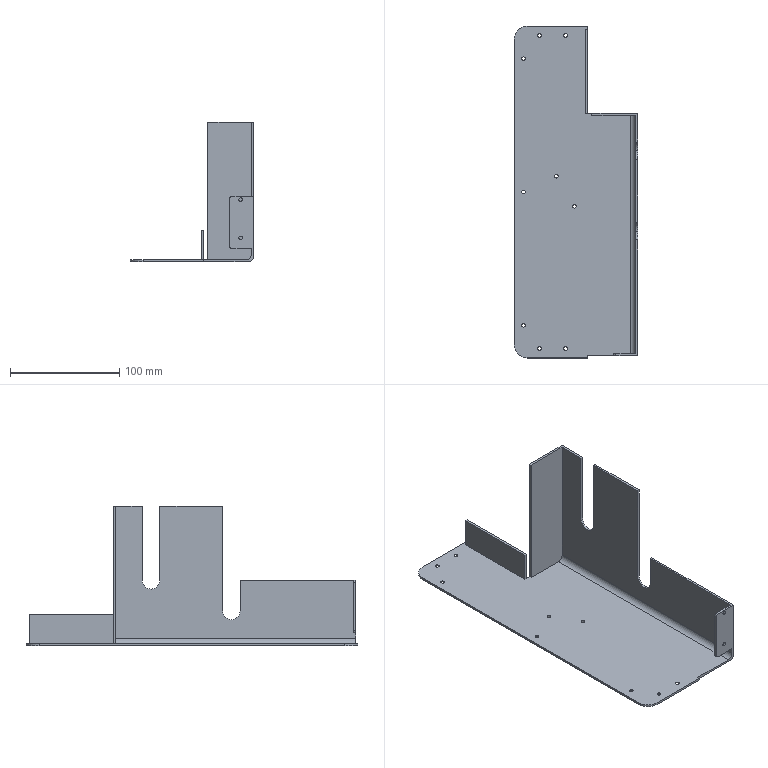Part | STEP file | 11-FG-E03011 | 1 solid | 73 faces | box 113 x 304 x 128 mm | volume 112726 mm3 | cylinder 32 | plane 27 | cone 14 | commonest cylinder face diameters 3.4 x14 3.3 x8 16 x4 4 x2 10 x2 24 x2